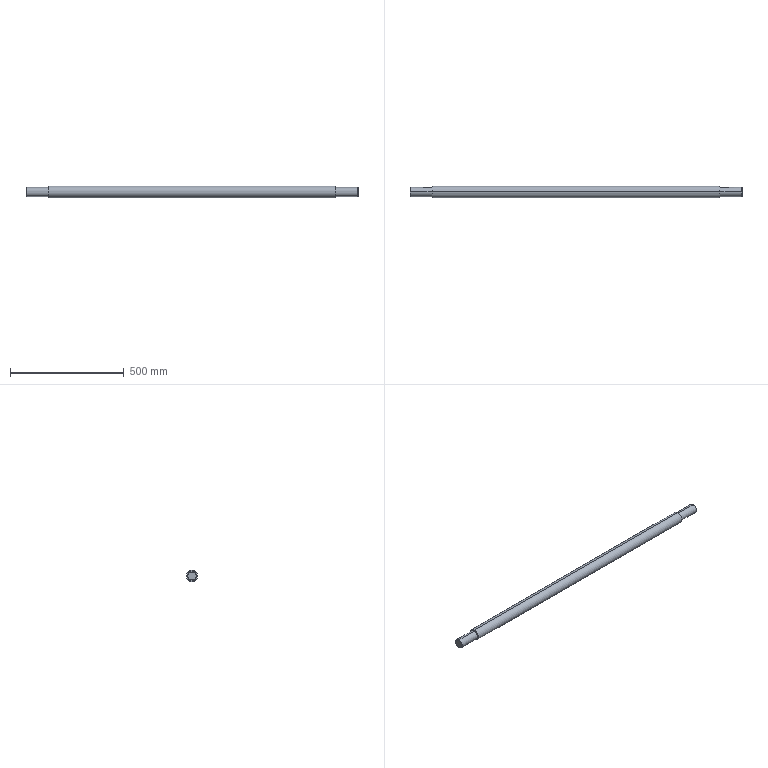Part | STEP file | Produce dryer mesh belt driven shaft | 1 solid | 24 faces | box 1461 x 50 x 50 mm | volume 2725239 mm3 | cylinder 10 | plane 10 | cone 4 | commonest cylinder face diameters 12 x4 40 x4 50 x2
STEP:
#1=CARTESIAN_POINT('',(-730.25,0.,18.));
#2=VERTEX_POINT('',#1);
#3=CARTESIAN_POINT('',(-730.25,0.,-18.));
#4=VERTEX_POINT('',#3);
#5=CARTESIAN_POINT('',(-730.25,0.,0.));
#6=DIRECTION('',(-1.,0.,0.));
#7=DIRECTION('',(0.,0.,-1.));
#8=AXIS2_PLACEMENT_3D('',#5,#6,#7);
#9=CIRCLE('',#8,18.);
#10=EDGE_CURVE('',#2,#4,#9,.T.);
#11=ORIENTED_EDGE('',*,*,#10,.F.);
#12=CARTESIAN_POINT('',(-728.25,0.,20.));
#13=VERTEX_POINT('',#12);
#14=CARTESIAN_POINT('',(-730.25,0.,18.));
#15=DIRECTION('',(0.7071,0.,0.7071));
#16=VECTOR('',#15,1000.);
#17=LINE('',#14,#16);
#18=EDGE_CURVE('',#2,#13,#17,.T.);
#19=ORIENTED_EDGE('',*,*,#18,.T.);
#20=CARTESIAN_POINT('',(-728.25,0.,-20.));
#21=VERTEX_POINT('',#20);
#22=CARTESIAN_POINT('',(-728.25,0.,0.));
#23=DIRECTION('',(1.,0.,0.));
#24=DIRECTION('',(0.,0.,-1.));
#25=AXIS2_PLACEMENT_3D('',#22,#23,#24);
#26=CIRCLE('',#25,20.);
#27=EDGE_CURVE('',#21,#13,#26,.T.);
#28=ORIENTED_EDGE('',*,*,#27,.F.);
#29=CARTESIAN_POINT('',(-730.25,0.,-18.));
#30=DIRECTION('',(0.7071,0.,-0.7071));
#31=VECTOR('',#30,1000.);
#32=LINE('',#29,#31);
#33=EDGE_CURVE('',#4,#21,#32,.T.);
#34=ORIENTED_EDGE('',*,*,#33,.F.);
#35=EDGE_LOOP('',(#11,#19,#28,#34));
#36=FACE_OUTER_BOUND('',#35,.T.);
#37=CARTESIAN_POINT('',(-730.25,0.,0.));
#38=DIRECTION('',(1.,0.,0.));
#39=DIRECTION('',(0.,0.,-1.));
#40=AXIS2_PLACEMENT_3D('',#37,#38,#39);
#41=CONICAL_SURFACE('',#40,18.,0.7854);
#42=ADVANCED_FACE('',(#36),#41,.T.);
#43=CARTESIAN_POINT('',(730.25,0.,-18.));
#44=VERTEX_POINT('',#43);
#45=CARTESIAN_POINT('',(730.25,0.,18.));
#46=VERTEX_POINT('',#45);
#47=CARTESIAN_POINT('',(730.25,0.,0.));
#48=DIRECTION('',(1.,0.,0.));
#49=DIRECTION('',(0.,0.,1.));
#50=AXIS2_PLACEMENT_3D('',#47,#48,#49);
#51=CIRCLE('',#50,18.);
#52=EDGE_CURVE('',#44,#46,#51,.T.);
#53=ORIENTED_EDGE('',*,*,#52,.F.);
#54=CARTESIAN_POINT('',(728.25,0.,-20.));
#55=VERTEX_POINT('',#54);
#56=CARTESIAN_POINT('',(728.25,0.,-20.));
#57=DIRECTION('',(-0.7071,0.,-0.7071));
#58=VECTOR('',#57,1000.);
#59=LINE('',#56,#58);
#60=EDGE_CURVE('',#44,#55,#59,.T.);
#61=ORIENTED_EDGE('',*,*,#60,.T.);
#62=CARTESIAN_POINT('',(728.25,0.,20.));
#63=VERTEX_POINT('',#62);
#64=CARTESIAN_POINT('',(728.25,0.,0.));
#65=DIRECTION('',(-1.,0.,0.));
#66=DIRECTION('',(0.,0.,1.));
#67=AXIS2_PLACEMENT_3D('',#64,#65,#66);
#68=CIRCLE('',#67,20.);
#69=EDGE_CURVE('',#63,#55,#68,.T.);
#70=ORIENTED_EDGE('',*,*,#69,.F.);
#71=CARTESIAN_POINT('',(728.25,0.,20.));
#72=DIRECTION('',(-0.7071,0.,0.7071));
#73=VECTOR('',#72,1000.);
#74=LINE('',#71,#73);
#75=EDGE_CURVE('',#46,#63,#74,.T.);
#76=ORIENTED_EDGE('',*,*,#75,.F.);
#77=EDGE_LOOP('',(#53,#61,#70,#76));
#78=FACE_OUTER_BOUND('',#77,.T.);
#79=CARTESIAN_POINT('',(728.25,0.,0.));
#80=DIRECTION('',(-1.,0.,0.));
#81=DIRECTION('',(0.,0.,1.));
#82=AXIS2_PLACEMENT_3D('',#79,#80,#81);
#83=CONICAL_SURFACE('',#82,20.,0.7854);
#84=ADVANCED_FACE('',(#78),#83,.T.);
#85=CARTESIAN_POINT('',(-667.75,19.079,-6.));
#86=VERTEX_POINT('',#85);
#87=CARTESIAN_POINT('',(-640.75,19.079,-6.));
#88=VERTEX_POINT('',#87);
#89=CARTESIAN_POINT('',(-730.25,19.079,-6.));
#90=DIRECTION('',(1.,0.,0.));
#91=VECTOR('',#90,1000.);
#92=LINE('',#89,#91);
#93=EDGE_CURVE('',#86,#88,#92,.T.);
#94=ORIENTED_EDGE('',*,*,#93,.T.);
#95=CARTESIAN_POINT('',(-640.75,19.079,6.));
#96=VERTEX_POINT('',#95);
#97=CARTESIAN_POINT('',(-640.75,19.079,-6.));
#98=CARTESIAN_POINT('',(-640.357,19.079,-6.));
#99=CARTESIAN_POINT('',(-639.963,19.091,-5.961));
#100=CARTESIAN_POINT('',(-639.184,19.139,-5.806));
#101=CARTESIAN_POINT('',(-638.809,19.174,-5.691));
#102=CARTESIAN_POINT('',(-638.086,19.261,-5.39));
#103=CARTESIAN_POINT('',(-637.735,19.313,-5.202));
#104=CARTESIAN_POINT('',(-637.086,19.425,-4.767));
#105=CARTESIAN_POINT('',(-636.785,19.484,-4.521));
#106=CARTESIAN_POINT('',(-636.37,19.575,-4.105));
#107=CARTESIAN_POINT('',(-636.237,19.605,-3.959));
#108=CARTESIAN_POINT('',(-635.989,19.664,-3.657));
#109=CARTESIAN_POINT('',(-635.873,19.692,-3.5));
#110=CARTESIAN_POINT('',(-635.548,19.774,-3.015));
#111=CARTESIAN_POINT('',(-635.362,19.824,-2.67));
#112=CARTESIAN_POINT('',(-635.058,19.909,-1.939));
#113=CARTESIAN_POINT('',(-634.944,19.943,-1.564));
#114=CARTESIAN_POINT('',(-634.828,19.977,-0.9868));
#115=CARTESIAN_POINT('',(-634.799,19.985,-0.7922));
#116=CARTESIAN_POINT('',(-634.76,19.997,-0.398));
#117=CARTESIAN_POINT('',(-634.75,20.,-0.1981));
#118=CARTESIAN_POINT('',(-634.75,20.,0.3951));
#119=CARTESIAN_POINT('',(-634.789,19.988,0.7861));
#120=CARTESIAN_POINT('',(-634.904,19.954,1.366));
#121=CARTESIAN_POINT('',(-634.953,19.94,1.559));
#122=CARTESIAN_POINT('',(-635.068,19.907,1.938));
#123=CARTESIAN_POINT('',(-635.135,19.888,2.123));
#124=CARTESIAN_POINT('',(-635.36,19.825,2.665));
#125=CARTESIAN_POINT('',(-635.545,19.775,3.01));
#126=CARTESIAN_POINT('',(-635.984,19.664,3.666));
#127=CARTESIAN_POINT('',(-636.231,19.605,3.967));
#128=CARTESIAN_POINT('',(-636.644,19.515,4.379));
#129=CARTESIAN_POINT('',(-636.788,19.485,4.51));
#130=CARTESIAN_POINT('',(-637.091,19.426,4.759));
#131=CARTESIAN_POINT('',(-637.25,19.397,4.877));
#132=CARTESIAN_POINT('',(-637.738,19.312,5.204));
#133=CARTESIAN_POINT('',(-638.081,19.261,5.388));
#134=CARTESIAN_POINT('',(-638.804,19.174,5.689));
#135=CARTESIAN_POINT('',(-639.187,19.139,5.806));
#136=CARTESIAN_POINT('',(-639.959,19.091,5.961));
#137=CARTESIAN_POINT('',(-640.351,19.079,6.));
#138=CARTESIAN_POINT('',(-640.75,19.079,6.));
#139=B_SPLINE_CURVE_WITH_KNOTS('',3,(#97,#98,#99,#100,#101,#102,#103,#104,#105,#106,#107,#108,#109,#110,#111,#112,#113,#114,#115,#116,#117,#118,#119,#120,#121,#122,#123,#124,#125,#126,#127,#128,#129,#130,#131,#132,#133,#134,#135,#136,#137,#138),.UNSPECIFIED.,.F.,.F.,(4,2,2,2,2,2,2,2,2,2,2,2,2,2,2,2,2,2,2,2,4),(0.01887,0.02005,0.02123,0.0224,0.02358,0.02417,0.02476,0.02594,0.02712,0.02771,0.0283,0.02948,0.03007,0.03066,0.03184,0.03301,0.0336,0.03419,0.03537,0.03655,0.03773),.UNSPECIFIED.);
#140=EDGE_CURVE('',#88,#96,#139,.T.);
#141=ORIENTED_EDGE('',*,*,#140,.T.);
#142=CARTESIAN_POINT('',(-667.75,19.079,6.));
#143=VERTEX_POINT('',#142);
#144=CARTESIAN_POINT('',(-730.25,19.079,6.));
#145=DIRECTION('',(-1.,0.,0.));
#146=VECTOR('',#145,1000.);
#147=LINE('',#144,#146);
#148=EDGE_CURVE('',#96,#143,#147,.T.);
#149=ORIENTED_EDGE('',*,*,#148,.T.);
#150=CARTESIAN_POINT('',(-667.75,19.079,6.));
#151=CARTESIAN_POINT('',(-668.149,19.079,6.));
#152=CARTESIAN_POINT('',(-668.54,19.091,5.961));
#153=CARTESIAN_POINT('',(-669.118,19.127,5.845));
#154=CARTESIAN_POINT('',(-669.308,19.141,5.797));
#155=CARTESIAN_POINT('',(-669.686,19.176,5.682));
#156=CARTESIAN_POINT('',(-669.874,19.196,5.615));
#157=CARTESIAN_POINT('',(-670.418,19.261,5.389));
#158=CARTESIAN_POINT('',(-670.761,19.312,5.204));
#159=CARTESIAN_POINT('',(-671.249,19.396,4.878));
#160=CARTESIAN_POINT('',(-671.408,19.426,4.76));
#161=CARTESIAN_POINT('',(-671.711,19.485,4.511));
#162=CARTESIAN_POINT('',(-671.855,19.515,4.38));
#163=CARTESIAN_POINT('',(-672.267,19.604,3.968));
#164=CARTESIAN_POINT('',(-672.515,19.664,3.668));
#165=CARTESIAN_POINT('',(-672.954,19.775,3.013));
#166=CARTESIAN_POINT('',(-673.139,19.825,2.667));
#167=CARTESIAN_POINT('',(-673.364,19.887,2.127));
#168=CARTESIAN_POINT('',(-673.43,19.906,1.942));
#169=CARTESIAN_POINT('',(-673.545,19.94,1.566));
#170=CARTESIAN_POINT('',(-673.594,19.954,1.372));
#171=CARTESIAN_POINT('',(-673.711,19.988,0.7905));
#172=CARTESIAN_POINT('',(-673.75,20.,0.3997));
#173=CARTESIAN_POINT('',(-673.75,20.,-0.3879));
#174=CARTESIAN_POINT('',(-673.711,19.988,-0.788));
#175=CARTESIAN_POINT('',(-673.557,19.943,-1.559));
#176=CARTESIAN_POINT('',(-673.443,19.91,-1.935));
#177=CARTESIAN_POINT('',(-673.216,19.846,-2.482));
#178=CARTESIAN_POINT('',(-673.131,19.823,-2.661));
#179=CARTESIAN_POINT('',(-672.946,19.774,-3.006));
#180=CARTESIAN_POINT('',(-672.846,19.747,-3.173));
#181=CARTESIAN_POINT('',(-672.629,19.693,-3.497));
#182=CARTESIAN_POINT('',(-672.513,19.664,-3.654));
#183=CARTESIAN_POINT('',(-672.265,19.605,-3.956));
#184=CARTESIAN_POINT('',(-672.132,19.575,-4.103));
#185=CARTESIAN_POINT('',(-671.717,19.485,-4.518));
#186=CARTESIAN_POINT('',(-671.417,19.425,-4.765));
#187=CARTESIAN_POINT('',(-670.769,19.314,-5.2));
#188=CARTESIAN_POINT('',(-670.418,19.261,-5.388));
#189=CARTESIAN_POINT('',(-669.696,19.174,-5.689));
#190=CARTESIAN_POINT('',(-669.322,19.14,-5.804));
#191=CARTESIAN_POINT('',(-668.548,19.092,-5.96));
#192=CARTESIAN_POINT('',(-668.149,19.079,-6.));
#193=CARTESIAN_POINT('',(-667.75,19.079,-6.));
#194=B_SPLINE_CURVE_WITH_KNOTS('',3,(#150,#151,#152,#153,#154,#155,#156,#157,#158,#159,#160,#161,#162,#163,#164,#165,#166,#167,#168,#169,#170,#171,#172,#173,#174,#175,#176,#177,#178,#179,#180,#181,#182,#183,#184,#185,#186,#187,#188,#189,#190,#191,#192,#193),.UNSPECIFIED.,.F.,.F.,(4,2,2,2,2,2,2,2,2,2,2,2,2,2,2,2,2,2,2,2,2,4),(0.,0.001179,0.001768,0.002358,0.003536,0.004126,0.004715,0.005894,0.007073,0.007662,0.008252,0.009431,0.01061,0.01179,0.01238,0.01297,0.01356,0.01415,0.01532,0.0165,0.01768,0.01886),.UNSPECIFIED.);
#195=EDGE_CURVE('',#143,#86,#194,.T.);
#196=ORIENTED_EDGE('',*,*,#195,.T.);
#197=EDGE_LOOP('',(#94,#141,#149,#196));
#198=FACE_BOUND('',#197,.T.);
#199=CARTESIAN_POINT('',(-632.75,0.,20.));
#200=VERTEX_POINT('',#199);
#201=CARTESIAN_POINT('',(-632.75,0.,-20.));
#202=VERTEX_POINT('',#201);
#203=CARTESIAN_POINT('',(-632.75,0.,0.));
#204=DIRECTION('',(-1.,0.,0.));
#205=DIRECTION('',(0.,0.,1.));
#206=AXIS2_PLACEMENT_3D('',#203,#204,#205);
#207=CIRCLE('',#206,20.);
#208=EDGE_CURVE('',#200,#202,#207,.T.);
#209=ORIENTED_EDGE('',*,*,#208,.T.);
#210=CARTESIAN_POINT('',(-730.25,0.,-20.));
#211=DIRECTION('',(-1.,0.,0.));
#212=VECTOR('',#211,1000.);
#213=LINE('',#210,#212);
#214=EDGE_CURVE('',#202,#21,#213,.T.);
#215=ORIENTED_EDGE('',*,*,#214,.T.);
#216=ORIENTED_EDGE('',*,*,#27,.T.);
#217=CARTESIAN_POINT('',(-730.25,0.,20.));
#218=DIRECTION('',(-1.,0.,0.));
#219=VECTOR('',#218,1000.);
#220=LINE('',#217,#219);
#221=EDGE_CURVE('',#200,#13,#220,.T.);
#222=ORIENTED_EDGE('',*,*,#221,.F.);
#223=EDGE_LOOP('',(#209,#215,#216,#222));
#224=FACE_OUTER_BOUND('',#223,.T.);
#225=CARTESIAN_POINT('',(-730.25,0.,0.));
#226=DIRECTION('',(-1.,0.,0.));
#227=DIRECTION('',(0.,0.,1.));
#228=AXIS2_PLACEMENT_3D('',#225,#226,#227);
#229=CYLINDRICAL_SURFACE('',#228,20.);
#230=ADVANCED_FACE('',(#198,#224),#229,.T.);
#231=CARTESIAN_POINT('',(632.75,0.,25.));
#232=VERTEX_POINT('',#231);
#233=CARTESIAN_POINT('',(632.75,0.,-25.));
#234=VERTEX_POINT('',#233);
#235=CARTESIAN_POINT('',(632.75,0.,0.));
#236=DIRECTION('',(-1.,0.,0.));
#237=DIRECTION('',(0.,0.,1.));
#238=AXIS2_PLACEMENT_3D('',#235,#236,#237);
#239=CIRCLE('',#238,25.);
#240=EDGE_CURVE('',#232,#234,#239,.T.);
#241=ORIENTED_EDGE('',*,*,#240,.T.);
#242=CARTESIAN_POINT('',(-632.75,0.,-25.));
#243=VERTEX_POINT('',#242);
#244=CARTESIAN_POINT('',(-730.25,0.,-25.));
#245=DIRECTION('',(-1.,0.,0.));
#246=VECTOR('',#245,1000.);
#247=LINE('',#244,#246);
#248=EDGE_CURVE('',#234,#243,#247,.T.);
#249=ORIENTED_EDGE('',*,*,#248,.T.);
#250=CARTESIAN_POINT('',(-632.75,0.,25.));
#251=VERTEX_POINT('',#250);
#252=CARTESIAN_POINT('',(-632.75,0.,0.));
#253=DIRECTION('',(-1.,0.,0.));
#254=DIRECTION('',(0.,0.,1.));
#255=AXIS2_PLACEMENT_3D('',#252,#253,#254);
#256=CIRCLE('',#255,25.);
#257=EDGE_CURVE('',#251,#243,#256,.T.);
#258=ORIENTED_EDGE('',*,*,#257,.F.);
#259=CARTESIAN_POINT('',(-730.25,0.,25.));
#260=DIRECTION('',(-1.,0.,0.));
#261=VECTOR('',#260,1000.);
#262=LINE('',#259,#261);
#263=EDGE_CURVE('',#232,#251,#262,.T.);
#264=ORIENTED_EDGE('',*,*,#263,.F.);
#265=EDGE_LOOP('',(#241,#249,#258,#264));
#266=FACE_OUTER_BOUND('',#265,.T.);
#267=CARTESIAN_POINT('',(-730.25,0.,0.));
#268=DIRECTION('',(-1.,0.,0.));
#269=DIRECTION('',(0.,0.,1.));
#270=AXIS2_PLACEMENT_3D('',#267,#268,#269);
#271=CYLINDRICAL_SURFACE('',#270,25.);
#272=ADVANCED_FACE('',(#266),#271,.T.);
#273=CARTESIAN_POINT('',(667.75,19.079,6.));
#274=VERTEX_POINT('',#273);
#275=CARTESIAN_POINT('',(640.75,19.079,6.));
#276=VERTEX_POINT('',#275);
#277=CARTESIAN_POINT('',(-730.25,19.079,6.));
#278=DIRECTION('',(-1.,0.,0.));
#279=VECTOR('',#278,1000.);
#280=LINE('',#277,#279);
#281=EDGE_CURVE('',#274,#276,#280,.T.);
#282=ORIENTED_EDGE('',*,*,#281,.T.);
#283=CARTESIAN_POINT('',(640.75,19.079,-6.));
#284=VERTEX_POINT('',#283);
#285=CARTESIAN_POINT('',(640.75,19.079,6.));
#286=CARTESIAN_POINT('',(640.351,19.079,6.));
#287=CARTESIAN_POINT('',(639.96,19.091,5.961));
#288=CARTESIAN_POINT('',(639.382,19.127,5.845));
#289=CARTESIAN_POINT('',(639.192,19.141,5.797));
#290=CARTESIAN_POINT('',(638.814,19.176,5.682));
#291=CARTESIAN_POINT('',(638.626,19.196,5.615));
#292=CARTESIAN_POINT('',(638.082,19.261,5.389));
#293=CARTESIAN_POINT('',(637.739,19.312,5.204));
#294=CARTESIAN_POINT('',(637.251,19.396,4.878));
#295=CARTESIAN_POINT('',(637.092,19.426,4.76));
#296=CARTESIAN_POINT('',(636.789,19.485,4.511));
#297=CARTESIAN_POINT('',(636.645,19.515,4.38));
#298=CARTESIAN_POINT('',(636.233,19.604,3.968));
#299=CARTESIAN_POINT('',(635.985,19.664,3.668));
#300=CARTESIAN_POINT('',(635.546,19.775,3.013));
#301=CARTESIAN_POINT('',(635.361,19.825,2.667));
#302=CARTESIAN_POINT('',(635.136,19.887,2.127));
#303=CARTESIAN_POINT('',(635.07,19.906,1.942));
#304=CARTESIAN_POINT('',(634.955,19.94,1.566));
#305=CARTESIAN_POINT('',(634.906,19.954,1.372));
#306=CARTESIAN_POINT('',(634.789,19.988,0.7905));
#307=CARTESIAN_POINT('',(634.75,20.,0.3997));
#308=CARTESIAN_POINT('',(634.75,20.,-0.3879));
#309=CARTESIAN_POINT('',(634.789,19.988,-0.788));
#310=CARTESIAN_POINT('',(634.943,19.943,-1.559));
#311=CARTESIAN_POINT('',(635.057,19.91,-1.935));
#312=CARTESIAN_POINT('',(635.284,19.846,-2.482));
#313=CARTESIAN_POINT('',(635.369,19.823,-2.661));
#314=CARTESIAN_POINT('',(635.554,19.774,-3.006));
#315=CARTESIAN_POINT('',(635.654,19.747,-3.173));
#316=CARTESIAN_POINT('',(635.871,19.693,-3.497));
#317=CARTESIAN_POINT('',(635.987,19.664,-3.654));
#318=CARTESIAN_POINT('',(636.235,19.605,-3.956));
#319=CARTESIAN_POINT('',(636.368,19.575,-4.103));
#320=CARTESIAN_POINT('',(636.783,19.485,-4.518));
#321=CARTESIAN_POINT('',(637.083,19.425,-4.765));
#322=CARTESIAN_POINT('',(637.731,19.314,-5.2));
#323=CARTESIAN_POINT('',(638.082,19.261,-5.388));
#324=CARTESIAN_POINT('',(638.804,19.174,-5.689));
#325=CARTESIAN_POINT('',(639.178,19.14,-5.804));
#326=CARTESIAN_POINT('',(639.952,19.092,-5.96));
#327=CARTESIAN_POINT('',(640.351,19.079,-6.));
#328=CARTESIAN_POINT('',(640.75,19.079,-6.));
#329=B_SPLINE_CURVE_WITH_KNOTS('',3,(#285,#286,#287,#288,#289,#290,#291,#292,#293,#294,#295,#296,#297,#298,#299,#300,#301,#302,#303,#304,#305,#306,#307,#308,#309,#310,#311,#312,#313,#314,#315,#316,#317,#318,#319,#320,#321,#322,#323,#324,#325,#326,#327,#328),.UNSPECIFIED.,.F.,.F.,(4,2,2,2,2,2,2,2,2,2,2,2,2,2,2,2,2,2,2,2,2,4),(0.,0.001179,0.001768,0.002358,0.003536,0.004126,0.004715,0.005894,0.007073,0.007662,0.008252,0.009431,0.01061,0.01179,0.01238,0.01297,0.01356,0.01415,0.01532,0.0165,0.01768,0.01886),.UNSPECIFIED.);
#330=EDGE_CURVE('',#276,#284,#329,.T.);
#331=ORIENTED_EDGE('',*,*,#330,.T.);
#332=CARTESIAN_POINT('',(667.75,19.079,-6.));
#333=VERTEX_POINT('',#332);
#334=CARTESIAN_POINT('',(-730.25,19.079,-6.));
#335=DIRECTION('',(1.,0.,0.));
#336=VECTOR('',#335,1000.);
#337=LINE('',#334,#336);
#338=EDGE_CURVE('',#284,#333,#337,.T.);
#339=ORIENTED_EDGE('',*,*,#338,.T.);
#340=CARTESIAN_POINT('',(667.75,19.079,-6.));
#341=CARTESIAN_POINT('',(668.143,19.079,-6.));
#342=CARTESIAN_POINT('',(668.537,19.091,-5.961));
#343=CARTESIAN_POINT('',(669.316,19.139,-5.806));
#344=CARTESIAN_POINT('',(669.691,19.174,-5.691));
#345=CARTESIAN_POINT('',(670.414,19.261,-5.39));
#346=CARTESIAN_POINT('',(670.765,19.313,-5.202));
#347=CARTESIAN_POINT('',(671.414,19.425,-4.767));
#348=CARTESIAN_POINT('',(671.715,19.484,-4.521));
#349=CARTESIAN_POINT('',(672.13,19.575,-4.105));
#350=CARTESIAN_POINT('',(672.263,19.605,-3.959));
#351=CARTESIAN_POINT('',(672.511,19.664,-3.657));
#352=CARTESIAN_POINT('',(672.627,19.692,-3.5));
#353=CARTESIAN_POINT('',(672.952,19.774,-3.015));
#354=CARTESIAN_POINT('',(673.138,19.824,-2.67));
#355=CARTESIAN_POINT('',(673.442,19.909,-1.939));
#356=CARTESIAN_POINT('',(673.556,19.943,-1.564));
#357=CARTESIAN_POINT('',(673.672,19.977,-0.9868));
#358=CARTESIAN_POINT('',(673.701,19.985,-0.7922));
#359=CARTESIAN_POINT('',(673.74,19.997,-0.398));
#360=CARTESIAN_POINT('',(673.75,20.,-0.1981));
#361=CARTESIAN_POINT('',(673.75,20.,0.3951));
#362=CARTESIAN_POINT('',(673.711,19.988,0.7861));
#363=CARTESIAN_POINT('',(673.596,19.954,1.366));
#364=CARTESIAN_POINT('',(673.547,19.94,1.559));
#365=CARTESIAN_POINT('',(673.432,19.907,1.938));
#366=CARTESIAN_POINT('',(673.365,19.888,2.123));
#367=CARTESIAN_POINT('',(673.14,19.825,2.665));
#368=CARTESIAN_POINT('',(672.955,19.775,3.01));
#369=CARTESIAN_POINT('',(672.516,19.664,3.666));
#370=CARTESIAN_POINT('',(672.269,19.605,3.967));
#371=CARTESIAN_POINT('',(671.856,19.515,4.379));
#372=CARTESIAN_POINT('',(671.712,19.485,4.51));
#373=CARTESIAN_POINT('',(671.409,19.426,4.759));
#374=CARTESIAN_POINT('',(671.25,19.397,4.877));
#375=CARTESIAN_POINT('',(670.762,19.312,5.204));
#376=CARTESIAN_POINT('',(670.419,19.261,5.388));
#377=CARTESIAN_POINT('',(669.696,19.174,5.689));
#378=CARTESIAN_POINT('',(669.313,19.139,5.806));
#379=CARTESIAN_POINT('',(668.541,19.091,5.961));
#380=CARTESIAN_POINT('',(668.149,19.079,6.));
#381=CARTESIAN_POINT('',(667.75,19.079,6.));
#382=B_SPLINE_CURVE_WITH_KNOTS('',3,(#340,#341,#342,#343,#344,#345,#346,#347,#348,#349,#350,#351,#352,#353,#354,#355,#356,#357,#358,#359,#360,#361,#362,#363,#364,#365,#366,#367,#368,#369,#370,#371,#372,#373,#374,#375,#376,#377,#378,#379,#380,#381),.UNSPECIFIED.,.F.,.F.,(4,2,2,2,2,2,2,2,2,2,2,2,2,2,2,2,2,2,2,2,4),(0.01887,0.02005,0.02123,0.0224,0.02358,0.02417,0.02476,0.02594,0.02712,0.02771,0.0283,0.02948,0.03007,0.03066,0.03184,0.03301,0.0336,0.03419,0.03537,0.03655,0.03773),.UNSPECIFIED.);
#383=EDGE_CURVE('',#333,#274,#382,.T.);
#384=ORIENTED_EDGE('',*,*,#383,.T.);
#385=EDGE_LOOP('',(#282,#331,#339,#384));
#386=FACE_BOUND('',#385,.T.);
#387=ORIENTED_EDGE('',*,*,#69,.T.);
#388=CARTESIAN_POINT('',(632.75,0.,-20.));
#389=VERTEX_POINT('',#388);
#390=CARTESIAN_POINT('',(-730.25,0.,-20.));
#391=DIRECTION('',(-1.,0.,0.));
#392=VECTOR('',#391,1000.);
#393=LINE('',#390,#392);
#394=EDGE_CURVE('',#55,#389,#393,.T.);
#395=ORIENTED_EDGE('',*,*,#394,.T.);
#396=CARTESIAN_POINT('',(632.75,0.,20.));
#397=VERTEX_POINT('',#396);
#398=CARTESIAN_POINT('',(632.75,0.,0.));
#399=DIRECTION('',(-1.,0.,0.));
#400=DIRECTION('',(0.,0.,1.));
#401=AXIS2_PLACEMENT_3D('',#398,#399,#400);
#402=CIRCLE('',#401,20.);
#403=EDGE_CURVE('',#397,#389,#402,.T.);
#404=ORIENTED_EDGE('',*,*,#403,.F.);
#405=CARTESIAN_POINT('',(-730.25,0.,20.));
#406=DIRECTION('',(-1.,0.,0.));
#407=VECTOR('',#406,1000.);
#408=LINE('',#405,#407);
#409=EDGE_CURVE('',#63,#397,#408,.T.);
#410=ORIENTED_EDGE('',*,*,#409,.F.);
#411=EDGE_LOOP('',(#387,#395,#404,#410));
#412=FACE_OUTER_BOUND('',#411,.T.);
#413=CARTESIAN_POINT('',(-730.25,0.,0.));
#414=DIRECTION('',(-1.,0.,0.));
#415=DIRECTION('',(0.,0.,1.));
#416=AXIS2_PLACEMENT_3D('',#413,#414,#415);
#417=CYLINDRICAL_SURFACE('',#416,20.);
#418=ADVANCED_FACE('',(#386,#412),#417,.T.);
#419=CARTESIAN_POINT('',(730.25,0.,0.));
#420=DIRECTION('',(1.,0.,0.));
#421=DIRECTION('',(0.,0.,1.));
#422=AXIS2_PLACEMENT_3D('',#419,#420,#421);
#423=CIRCLE('',#422,18.);
#424=EDGE_CURVE('',#46,#44,#423,.T.);
#425=ORIENTED_EDGE('',*,*,#424,.T.);
#426=ORIENTED_EDGE('',*,*,#52,.T.);
#427=EDGE_LOOP('',(#425,#426));
#428=FACE_OUTER_BOUND('',#427,.T.);
#429=CARTESIAN_POINT('',(730.25,0.,0.));
#430=DIRECTION('',(-1.,0.,0.));
#431=DIRECTION('',(0.,0.,1.));
#432=AXIS2_PLACEMENT_3D('',#429,#430,#431);
#433=PLANE('',#432);
#434=ADVANCED_FACE('',(#428),#433,.F.);
#435=ORIENTED_EDGE('',*,*,#394,.F.);
#436=CARTESIAN_POINT('',(728.25,0.,0.));
#437=DIRECTION('',(-1.,0.,0.));
#438=DIRECTION('',(0.,0.,1.));
#439=AXIS2_PLACEMENT_3D('',#436,#437,#438);
#440=CIRCLE('',#439,20.);
#441=EDGE_CURVE('',#55,#63,#440,.T.);
#442=ORIENTED_EDGE('',*,*,#441,.T.);
#443=ORIENTED_EDGE('',*,*,#409,.T.);
#444=CARTESIAN_POINT('',(632.75,0.,0.));
#445=DIRECTION('',(-1.,0.,0.));
#446=DIRECTION('',(0.,0.,1.));
#447=AXIS2_PLACEMENT_3D('',#444,#445,#446);
#448=CIRCLE('',#447,20.);
#449=EDGE_CURVE('',#389,#397,#448,.T.);
#450=ORIENTED_EDGE('',*,*,#449,.F.);
#451=EDGE_LOOP('',(#435,#442,#443,#450));
#452=FACE_OUTER_BOUND('',#451,.T.);
#453=CARTESIAN_POINT('',(-730.25,0.,0.));
#454=DIRECTION('',(-1.,0.,0.));
#455=DIRECTION('',(0.,0.,1.));
#456=AXIS2_PLACEMENT_3D('',#453,#454,#455);
#457=CYLINDRICAL_SURFACE('',#456,20.);
#458=ADVANCED_FACE('',(#452),#457,.T.);
#459=ORIENTED_EDGE('',*,*,#240,.F.);
#460=CARTESIAN_POINT('',(632.75,0.,0.));
#461=DIRECTION('',(-1.,0.,0.));
#462=DIRECTION('',(0.,0.,1.));
#463=AXIS2_PLACEMENT_3D('',#460,#461,#462);
#464=CIRCLE('',#463,25.);
#465=EDGE_CURVE('',#234,#232,#464,.T.);
#466=ORIENTED_EDGE('',*,*,#465,.F.);
#467=EDGE_LOOP('',(#459,#466));
#468=FACE_OUTER_BOUND('',#467,.T.);
#469=ORIENTED_EDGE('',*,*,#403,.T.);
#470=ORIENTED_EDGE('',*,*,#449,.T.);
#471=EDGE_LOOP('',(#469,#470));
#472=FACE_BOUND('',#471,.T.);
#473=CARTESIAN_POINT('',(632.75,20.,0.));
#474=DIRECTION('',(-1.,0.,0.));
#475=DIRECTION('',(0.,0.,1.));
#476=AXIS2_PLACEMENT_3D('',#473,#474,#475);
#477=PLANE('',#476);
#478=ADVANCED_FACE('',(#468,#472),#477,.F.);
#479=ORIENTED_EDGE('',*,*,#248,.F.);
#480=ORIENTED_EDGE('',*,*,#465,.T.);
#481=ORIENTED_EDGE('',*,*,#263,.T.);
#482=CARTESIAN_POINT('',(-632.75,0.,0.));
#483=DIRECTION('',(-1.,0.,0.));
#484=DIRECTION('',(0.,0.,1.));
#485=AXIS2_PLACEMENT_3D('',#482,#483,#484);
#486=CIRCLE('',#485,25.);
#487=EDGE_CURVE('',#243,#251,#486,.T.);
#488=ORIENTED_EDGE('',*,*,#487,.F.);
#489=EDGE_LOOP('',(#479,#480,#481,#488));
#490=FACE_OUTER_BOUND('',#489,.T.);
#491=CARTESIAN_POINT('',(-730.25,0.,0.));
#492=DIRECTION('',(-1.,0.,0.));
#493=DIRECTION('',(0.,0.,1.));
#494=AXIS2_PLACEMENT_3D('',#491,#492,#493);
#495=CYLINDRICAL_SURFACE('',#494,25.);
#496=ADVANCED_FACE('',(#490),#495,.T.);
#497=ORIENTED_EDGE('',*,*,#208,.F.);
#498=CARTESIAN_POINT('',(-632.75,0.,0.));
#499=DIRECTION('',(-1.,0.,0.));
#500=DIRECTION('',(0.,0.,1.));
#501=AXIS2_PLACEMENT_3D('',#498,#499,#500);
#502=CIRCLE('',#501,20.);
#503=EDGE_CURVE('',#202,#200,#502,.T.);
#504=ORIENTED_EDGE('',*,*,#503,.F.);
#505=EDGE_LOOP('',(#497,#504));
#506=FACE_BOUND('',#505,.T.);
#507=ORIENTED_EDGE('',*,*,#257,.T.);
#508=ORIENTED_EDGE('',*,*,#487,.T.);
#509=EDGE_LOOP('',(#507,#508));
#510=FACE_OUTER_BOUND('',#509,.T.);
#511=CARTESIAN_POINT('',(-632.75,25.,0.));
#512=DIRECTION('',(1.,0.,0.));
#513=DIRECTION('',(0.,0.,-1.));
#514=AXIS2_PLACEMENT_3D('',#511,#512,#513);
#515=PLANE('',#514);
#516=ADVANCED_FACE('',(#506,#510),#515,.F.);
#517=ORIENTED_EDGE('',*,*,#214,.F.);
#518=ORIENTED_EDGE('',*,*,#503,.T.);
#519=ORIENTED_EDGE('',*,*,#221,.T.);
#520=CARTESIAN_POINT('',(-728.25,0.,0.));
#521=DIRECTION('',(1.,0.,0.));
#522=DIRECTION('',(0.,0.,-1.));
#523=AXIS2_PLACEMENT_3D('',#520,#521,#522);
#524=CIRCLE('',#523,20.);
#525=EDGE_CURVE('',#13,#21,#524,.T.);
#526=ORIENTED_EDGE('',*,*,#525,.T.);
#527=EDGE_LOOP('',(#517,#518,#519,#526));
#528=FACE_OUTER_BOUND('',#527,.T.);
#529=CARTESIAN_POINT('',(-730.25,0.,0.));
#530=DIRECTION('',(-1.,0.,0.));
#531=DIRECTION('',(0.,0.,1.));
#532=AXIS2_PLACEMENT_3D('',#529,#530,#531);
#533=CYLINDRICAL_SURFACE('',#532,20.);
#534=ADVANCED_FACE('',(#528),#533,.T.);
#535=CARTESIAN_POINT('',(-730.25,0.,0.));
#536=DIRECTION('',(-1.,0.,0.));
#537=DIRECTION('',(0.,0.,-1.));
#538=AXIS2_PLACEMENT_3D('',#535,#536,#537);
#539=CIRCLE('',#538,18.);
#540=EDGE_CURVE('',#4,#2,#539,.T.);
#541=ORIENTED_EDGE('',*,*,#540,.T.);
#542=ORIENTED_EDGE('',*,*,#10,.T.);
#543=EDGE_LOOP('',(#541,#542));
#544=FACE_OUTER_BOUND('',#543,.T.);
#545=CARTESIAN_POINT('',(-730.25,20.,0.));
#546=DIRECTION('',(1.,0.,0.));
#547=DIRECTION('',(0.,0.,-1.));
#548=AXIS2_PLACEMENT_3D('',#545,#546,#547);
#549=PLANE('',#548);
#550=ADVANCED_FACE('',(#544),#549,.F.);
#551=CARTESIAN_POINT('',(-667.75,15.,6.));
#552=VERTEX_POINT('',#551);
#553=CARTESIAN_POINT('',(-667.75,15.,6.));
#554=DIRECTION('',(0.,1.,0.));
#555=VECTOR('',#554,1000.);
#556=LINE('',#553,#555);
#557=EDGE_CURVE('',#552,#143,#556,.T.);
#558=ORIENTED_EDGE('',*,*,#557,.F.);
#559=CARTESIAN_POINT('',(-667.75,15.,-6.));
#560=VERTEX_POINT('',#559);
#561=CARTESIAN_POINT('',(-667.75,15.,0.));
#562=DIRECTION('',(0.,1.,0.));
#563=DIRECTION('',(0.,0.,1.));
#564=AXIS2_PLACEMENT_3D('',#561,#562,#563);
#565=CIRCLE('',#564,6.);
#566=EDGE_CURVE('',#560,#552,#565,.T.);
#567=ORIENTED_EDGE('',*,*,#566,.F.);
#568=CARTESIAN_POINT('',(-667.75,15.,-6.));
#569=DIRECTION('',(0.,1.,0.));
#570=VECTOR('',#569,1000.);
#571=LINE('',#568,#570);
#572=EDGE_CURVE('',#560,#86,#571,.T.);
#573=ORIENTED_EDGE('',*,*,#572,.T.);
#574=ORIENTED_EDGE('',*,*,#195,.F.);
#575=EDGE_LOOP('',(#558,#567,#573,#574));
#576=FACE_OUTER_BOUND('',#575,.T.);
#577=CARTESIAN_POINT('',(-667.75,15.,0.));
#578=DIRECTION('',(0.,1.,0.));
#579=DIRECTION('',(0.,0.,1.));
#580=AXIS2_PLACEMENT_3D('',#577,#578,#579);
#581=CYLINDRICAL_SURFACE('',#580,6.);
#582=ADVANCED_FACE('',(#576),#581,.F.);
#583=ORIENTED_EDGE('',*,*,#572,.F.);
#584=CARTESIAN_POINT('',(-640.75,15.,-6.));
#585=VERTEX_POINT('',#584);
#586=CARTESIAN_POINT('',(-667.75,15.,-6.));
#587=DIRECTION('',(-1.,0.,0.));
#588=VECTOR('',#587,1000.);
#589=LINE('',#586,#588);
#590=EDGE_CURVE('',#585,#560,#589,.T.);
#591=ORIENTED_EDGE('',*,*,#590,.F.);
#592=CARTESIAN_POINT('',(-640.75,15.,-6.));
#593=DIRECTION('',(0.,1.,0.));
#594=VECTOR('',#593,1000.);
#595=LINE('',#592,#594);
#596=EDGE_CURVE('',#585,#88,#595,.T.);
#597=ORIENTED_EDGE('',*,*,#596,.T.);
#598=ORIENTED_EDGE('',*,*,#93,.F.);
#599=EDGE_LOOP('',(#583,#591,#597,#598));
#600=FACE_OUTER_BOUND('',#599,.T.);
#601=CARTESIAN_POINT('',(-667.75,15.,-6.));
#602=DIRECTION('',(0.,0.,-1.));
#603=DIRECTION('',(-1.,0.,0.));
#604=AXIS2_PLACEMENT_3D('',#601,#602,#603);
#605=PLANE('',#604);
#606=ADVANCED_FACE('',(#600),#605,.F.);
#607=ORIENTED_EDGE('',*,*,#596,.F.);
#608=CARTESIAN_POINT('',(-640.75,15.,6.));
#609=VERTEX_POINT('',#608);
#610=CARTESIAN_POINT('',(-640.75,15.,0.));
#611=DIRECTION('',(0.,1.,0.));
#612=DIRECTION('',(0.,0.,1.));
#613=AXIS2_PLACEMENT_3D('',#610,#611,#612);
#614=CIRCLE('',#613,6.);
#615=EDGE_CURVE('',#609,#585,#614,.T.);
#616=ORIENTED_EDGE('',*,*,#615,.F.);
#617=CARTESIAN_POINT('',(-640.75,15.,6.));
#618=DIRECTION('',(0.,1.,0.));
#619=VECTOR('',#618,1000.);
#620=LINE('',#617,#619);
#621=EDGE_CURVE('',#609,#96,#620,.T.);
#622=ORIENTED_EDGE('',*,*,#621,.T.);
#623=ORIENTED_EDGE('',*,*,#140,.F.);
#624=EDGE_LOOP('',(#607,#616,#622,#623));
#625=FACE_OUTER_BOUND('',#624,.T.);
#626=CARTESIAN_POINT('',(-640.75,15.,0.));
#627=DIRECTION('',(0.,1.,0.));
#628=DIRECTION('',(0.,0.,1.));
#629=AXIS2_PLACEMENT_3D('',#626,#627,#628);
#630=CYLINDRICAL_SURFACE('',#629,6.);
#631=ADVANCED_FACE('',(#625),#630,.F.);
#632=ORIENTED_EDGE('',*,*,#621,.F.);
#633=CARTESIAN_POINT('',(-667.75,15.,6.));
#634=DIRECTION('',(1.,0.,0.));
#635=VECTOR('',#634,1000.);
#636=LINE('',#633,#635);
#637=EDGE_CURVE('',#552,#609,#636,.T.);
#638=ORIENTED_EDGE('',*,*,#637,.F.);
#639=ORIENTED_EDGE('',*,*,#557,.T.);
#640=ORIENTED_EDGE('',*,*,#148,.F.);
#641=EDGE_LOOP('',(#632,#638,#639,#640));
#642=FACE_OUTER_BOUND('',#641,.T.);
#643=CARTESIAN_POINT('',(-667.75,15.,6.));
#644=DIRECTION('',(0.,0.,1.));
#645=DIRECTION('',(1.,0.,0.));
#646=AXIS2_PLACEMENT_3D('',#643,#644,#645);
#647=PLANE('',#646);
#648=ADVANCED_FACE('',(#642),#647,.F.);
#649=ORIENTED_EDGE('',*,*,#566,.T.);
#650=ORIENTED_EDGE('',*,*,#637,.T.);
#651=ORIENTED_EDGE('',*,*,#615,.T.);
#652=ORIENTED_EDGE('',*,*,#590,.T.);
#653=EDGE_LOOP('',(#649,#650,#651,#652));
#654=FACE_OUTER_BOUND('',#653,.T.);
#655=CARTESIAN_POINT('',(-667.75,15.,0.));
#656=DIRECTION('',(0.,1.,0.));
#657=DIRECTION('',(0.,0.,1.));
#658=AXIS2_PLACEMENT_3D('',#655,#656,#657);
#659=PLANE('',#658);
#660=ADVANCED_FACE('',(#654),#659,.T.);
#661=CARTESIAN_POINT('',(667.75,15.,-6.));
#662=VERTEX_POINT('',#661);
#663=CARTESIAN_POINT('',(667.75,15.,-6.));
#664=DIRECTION('',(0.,1.,0.));
#665=VECTOR('',#664,1000.);
#666=LINE('',#663,#665);
#667=EDGE_CURVE('',#662,#333,#666,.T.);
#668=ORIENTED_EDGE('',*,*,#667,.F.);
#669=CARTESIAN_POINT('',(667.75,15.,6.));
#670=VERTEX_POINT('',#669);
#671=CARTESIAN_POINT('',(667.75,15.,0.));
#672=DIRECTION('',(0.,1.,0.));
#673=DIRECTION('',(0.,0.,-1.));
#674=AXIS2_PLACEMENT_3D('',#671,#672,#673);
#675=CIRCLE('',#674,6.);
#676=EDGE_CURVE('',#670,#662,#675,.T.);
#677=ORIENTED_EDGE('',*,*,#676,.F.);
#678=CARTESIAN_POINT('',(667.75,15.,6.));
#679=DIRECTION('',(0.,1.,0.));
#680=VECTOR('',#679,1000.);
#681=LINE('',#678,#680);
#682=EDGE_CURVE('',#670,#274,#681,.T.);
#683=ORIENTED_EDGE('',*,*,#682,.T.);
#684=ORIENTED_EDGE('',*,*,#383,.F.);
#685=EDGE_LOOP('',(#668,#677,#683,#684));
#686=FACE_OUTER_BOUND('',#685,.T.);
#687=CARTESIAN_POINT('',(667.75,15.,0.));
#688=DIRECTION('',(0.,1.,0.));
#689=DIRECTION('',(0.,0.,1.));
#690=AXIS2_PLACEMENT_3D('',#687,#688,#689);
#691=CYLINDRICAL_SURFACE('',#690,6.);
#692=ADVANCED_FACE('',(#686),#691,.F.);
#693=ORIENTED_EDGE('',*,*,#682,.F.);
#694=CARTESIAN_POINT('',(640.75,15.,6.));
#695=VERTEX_POINT('',#694);
#696=CARTESIAN_POINT('',(667.75,15.,6.));
#697=DIRECTION('',(1.,0.,0.));
#698=VECTOR('',#697,1000.);
#699=LINE('',#696,#698);
#700=EDGE_CURVE('',#695,#670,#699,.T.);
#701=ORIENTED_EDGE('',*,*,#700,.F.);
#702=CARTESIAN_POINT('',(640.75,15.,6.));
#703=DIRECTION('',(0.,1.,0.));
#704=VECTOR('',#703,1000.);
#705=LINE('',#702,#704);
#706=EDGE_CURVE('',#695,#276,#705,.T.);
#707=ORIENTED_EDGE('',*,*,#706,.T.);
#708=ORIENTED_EDGE('',*,*,#281,.F.);
#709=EDGE_LOOP('',(#693,#701,#707,#708));
#710=FACE_OUTER_BOUND('',#709,.T.);
#711=CARTESIAN_POINT('',(667.75,15.,6.));
#712=DIRECTION('',(0.,0.,1.));
#713=DIRECTION('',(1.,0.,0.));
#714=AXIS2_PLACEMENT_3D('',#711,#712,#713);
#715=PLANE('',#714);
#716=ADVANCED_FACE('',(#710),#715,.F.);
#717=ORIENTED_EDGE('',*,*,#706,.F.);
#718=CARTESIAN_POINT('',(640.75,15.,-6.));
#719=VERTEX_POINT('',#718);
#720=CARTESIAN_POINT('',(640.75,15.,0.));
#721=DIRECTION('',(0.,1.,0.));
#722=DIRECTION('',(0.,0.,-1.));
#723=AXIS2_PLACEMENT_3D('',#720,#721,#722);
#724=CIRCLE('',#723,6.);
#725=EDGE_CURVE('',#719,#695,#724,.T.);
#726=ORIENTED_EDGE('',*,*,#725,.F.);
#727=CARTESIAN_POINT('',(640.75,15.,-6.));
#728=DIRECTION('',(0.,1.,0.));
#729=VECTOR('',#728,1000.);
#730=LINE('',#727,#729);
#731=EDGE_CURVE('',#719,#284,#730,.T.);
#732=ORIENTED_EDGE('',*,*,#731,.T.);
#733=ORIENTED_EDGE('',*,*,#330,.F.);
#734=EDGE_LOOP('',(#717,#726,#732,#733));
#735=FACE_OUTER_BOUND('',#734,.T.);
#736=CARTESIAN_POINT('',(640.75,15.,0.));
#737=DIRECTION('',(0.,1.,0.));
#738=DIRECTION('',(0.,0.,1.));
#739=AXIS2_PLACEMENT_3D('',#736,#737,#738);
#740=CYLINDRICAL_SURFACE('',#739,6.);
#741=ADVANCED_FACE('',(#735),#740,.F.);
#742=ORIENTED_EDGE('',*,*,#731,.F.);
#743=CARTESIAN_POINT('',(667.75,15.,-6.));
#744=DIRECTION('',(-1.,0.,0.));
#745=VECTOR('',#744,1000.);
#746=LINE('',#743,#745);
#747=EDGE_CURVE('',#662,#719,#746,.T.);
#748=ORIENTED_EDGE('',*,*,#747,.F.);
#749=ORIENTED_EDGE('',*,*,#667,.T.);
#750=ORIENTED_EDGE('',*,*,#338,.F.);
#751=EDGE_LOOP('',(#742,#748,#749,#750));
#752=FACE_OUTER_BOUND('',#751,.T.);
#753=CARTESIAN_POINT('',(667.75,15.,-6.));
#754=DIRECTION('',(0.,0.,-1.));
#755=DIRECTION('',(-1.,0.,0.));
#756=AXIS2_PLACEMENT_3D('',#753,#754,#755);
#757=PLANE('',#756);
#758=ADVANCED_FACE('',(#752),#757,.F.);
#759=ORIENTED_EDGE('',*,*,#676,.T.);
#760=ORIENTED_EDGE('',*,*,#747,.T.);
#761=ORIENTED_EDGE('',*,*,#725,.T.);
#762=ORIENTED_EDGE('',*,*,#700,.T.);
#763=EDGE_LOOP('',(#759,#760,#761,#762));
#764=FACE_OUTER_BOUND('',#763,.T.);
#765=CARTESIAN_POINT('',(667.75,15.,0.));
#766=DIRECTION('',(0.,-1.,0.));
#767=DIRECTION('',(0.,0.,-1.));
#768=AXIS2_PLACEMENT_3D('',#765,#766,#767);
#769=PLANE('',#768);
#770=ADVANCED_FACE('',(#764),#769,.F.);
#771=ORIENTED_EDGE('',*,*,#60,.F.);
#772=ORIENTED_EDGE('',*,*,#424,.F.);
#773=ORIENTED_EDGE('',*,*,#75,.T.);
#774=ORIENTED_EDGE('',*,*,#441,.F.);
#775=EDGE_LOOP('',(#771,#772,#773,#774));
#776=FACE_OUTER_BOUND('',#775,.T.);
#777=CARTESIAN_POINT('',(728.25,0.,0.));
#778=DIRECTION('',(-1.,0.,0.));
#779=DIRECTION('',(0.,0.,1.));
#780=AXIS2_PLACEMENT_3D('',#777,#778,#779);
#781=CONICAL_SURFACE('',#780,20.,0.7854);
#782=ADVANCED_FACE('',(#776),#781,.T.);
#783=ORIENTED_EDGE('',*,*,#18,.F.);
#784=ORIENTED_EDGE('',*,*,#540,.F.);
#785=ORIENTED_EDGE('',*,*,#33,.T.);
#786=ORIENTED_EDGE('',*,*,#525,.F.);
#787=EDGE_LOOP('',(#783,#784,#785,#786));
#788=FACE_OUTER_BOUND('',#787,.T.);
#789=CARTESIAN_POINT('',(-730.25,0.,0.));
#790=DIRECTION('',(1.,0.,0.));
#791=DIRECTION('',(0.,0.,-1.));
#792=AXIS2_PLACEMENT_3D('',#789,#790,#791);
#793=CONICAL_SURFACE('',#792,18.,0.7854);
#794=ADVANCED_FACE('',(#788),#793,.T.);
#795=CLOSED_SHELL('',(#42,#84,#230,#272,#418,#434,#458,#478,#496,#516,#534,#550,#582,#606,#631,#648,#660,#692,#716,#741,#758,#770,#782,#794));
#796=MANIFOLD_SOLID_BREP('',#795);
#797=CARTESIAN_POINT('',(0.,0.,0.));
#798=DIRECTION('',(0.,0.,1.));
#799=DIRECTION('',(1.,0.,0.));
#800=AXIS2_PLACEMENT_3D('',#797,#798,#799);
#801=(LENGTH_UNIT()NAMED_UNIT(*)SI_UNIT(.MILLI.,.METRE.));
#802=UNCERTAINTY_MEASURE_WITH_UNIT(LENGTH_MEASURE(0.00001),#801,'','');
#803=(NAMED_UNIT(*)PLANE_ANGLE_UNIT()SI_UNIT($,.RADIAN.));
#804=(NAMED_UNIT(*)SI_UNIT($,.STERADIAN.)SOLID_ANGLE_UNIT());
#805=(GEOMETRIC_REPRESENTATION_CONTEXT(3)GLOBAL_UNCERTAINTY_ASSIGNED_CONTEXT((#802))GLOBAL_UNIT_ASSIGNED_CONTEXT((#801,#803,#804))REPRESENTATION_CONTEXT('',''));
#806=ADVANCED_BREP_SHAPE_REPRESENTATION('',(#796,#800),#805);